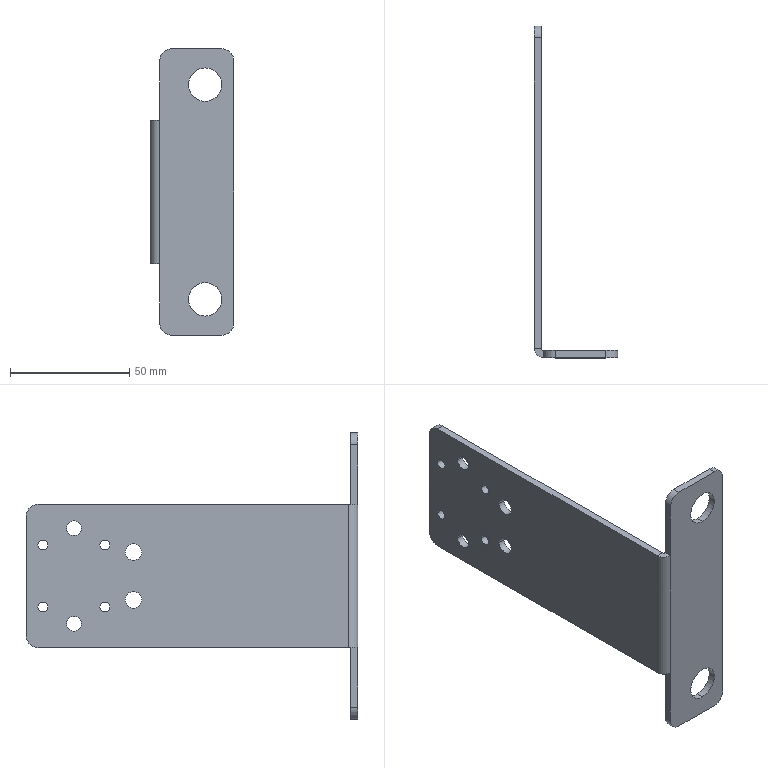Part | SolidWorks | features ICE 5, Fillet 2, ExtruThin 1, FlatPattern 1, FlattenBends 1, ProcessBends 1, SheetMetal 1 | 1 solid | 44 faces | box 35 x 139 x 120 mm | volume 34584 mm3 | cylinder 28 | plane 16 | commonest cylinder face diameters 4.2 x8 10 x6 6.2 x4 7 x4 14 x4 1.6 x1
STEP:
#1=CARTESIAN_POINT('',(0.,97.5,10.));
#2=VERTEX_POINT('',#1);
#3=CARTESIAN_POINT('',(0.,90.5,10.));
#4=VERTEX_POINT('',#3);
#5=CARTESIAN_POINT('',(0.,94.,10.));
#6=DIRECTION('',(-1.,0.,0.));
#7=DIRECTION('',(0.,-1.,0.));
#8=AXIS2_PLACEMENT_3D('',#5,#6,#7);
#9=CIRCLE('',#8,3.5);
#10=EDGE_CURVE('',#2,#4,#9,.T.);
#11=ORIENTED_EDGE('',*,*,#10,.T.);
#12=CARTESIAN_POINT('',(3.,90.5,10.));
#13=VERTEX_POINT('',#12);
#14=CARTESIAN_POINT('',(-7.,90.5,10.));
#15=DIRECTION('',(1.,0.,0.));
#16=VECTOR('',#15,1000.);
#17=LINE('',#14,#16);
#18=EDGE_CURVE('',#4,#13,#17,.T.);
#19=ORIENTED_EDGE('',*,*,#18,.T.);
#20=CARTESIAN_POINT('',(3.,97.5,10.));
#21=VERTEX_POINT('',#20);
#22=CARTESIAN_POINT('',(3.,94.,10.));
#23=DIRECTION('',(1.,0.,0.));
#24=DIRECTION('',(0.,1.,0.));
#25=AXIS2_PLACEMENT_3D('',#22,#23,#24);
#26=CIRCLE('',#25,3.5);
#27=EDGE_CURVE('',#13,#21,#26,.T.);
#28=ORIENTED_EDGE('',*,*,#27,.T.);
#29=CARTESIAN_POINT('',(-7.,97.5,10.));
#30=DIRECTION('',(1.,0.,0.));
#31=VECTOR('',#30,1000.);
#32=LINE('',#29,#31);
#33=EDGE_CURVE('',#2,#21,#32,.T.);
#34=ORIENTED_EDGE('',*,*,#33,.F.);
#35=EDGE_LOOP('',(#11,#19,#28,#34));
#36=FACE_OUTER_BOUND('',#35,.T.);
#37=CARTESIAN_POINT('',(-7.,94.,10.));
#38=DIRECTION('',(1.,0.,0.));
#39=DIRECTION('',(0.,1.,0.));
#40=AXIS2_PLACEMENT_3D('',#37,#38,#39);
#41=CYLINDRICAL_SURFACE('',#40,3.5);
#42=ADVANCED_FACE('',(#36),#41,.F.);
#43=CARTESIAN_POINT('',(0.,97.5,-10.));
#44=VERTEX_POINT('',#43);
#45=CARTESIAN_POINT('',(0.,90.5,-10.));
#46=VERTEX_POINT('',#45);
#47=CARTESIAN_POINT('',(0.,94.,-10.));
#48=DIRECTION('',(-1.,0.,0.));
#49=DIRECTION('',(0.,-1.,0.));
#50=AXIS2_PLACEMENT_3D('',#47,#48,#49);
#51=CIRCLE('',#50,3.5);
#52=EDGE_CURVE('',#44,#46,#51,.T.);
#53=ORIENTED_EDGE('',*,*,#52,.T.);
#54=CARTESIAN_POINT('',(3.,90.5,-10.));
#55=VERTEX_POINT('',#54);
#56=CARTESIAN_POINT('',(-7.,90.5,-10.));
#57=DIRECTION('',(1.,0.,0.));
#58=VECTOR('',#57,1000.);
#59=LINE('',#56,#58);
#60=EDGE_CURVE('',#46,#55,#59,.T.);
#61=ORIENTED_EDGE('',*,*,#60,.T.);
#62=CARTESIAN_POINT('',(3.,97.5,-10.));
#63=VERTEX_POINT('',#62);
#64=CARTESIAN_POINT('',(3.,94.,-10.));
#65=DIRECTION('',(1.,0.,0.));
#66=DIRECTION('',(0.,1.,0.));
#67=AXIS2_PLACEMENT_3D('',#64,#65,#66);
#68=CIRCLE('',#67,3.5);
#69=EDGE_CURVE('',#55,#63,#68,.T.);
#70=ORIENTED_EDGE('',*,*,#69,.T.);
#71=CARTESIAN_POINT('',(-7.,97.5,-10.));
#72=DIRECTION('',(1.,0.,0.));
#73=VECTOR('',#72,1000.);
#74=LINE('',#71,#73);
#75=EDGE_CURVE('',#44,#63,#74,.T.);
#76=ORIENTED_EDGE('',*,*,#75,.F.);
#77=EDGE_LOOP('',(#53,#61,#70,#76));
#78=FACE_OUTER_BOUND('',#77,.T.);
#79=CARTESIAN_POINT('',(-7.,94.,-10.));
#80=DIRECTION('',(1.,0.,0.));
#81=DIRECTION('',(0.,1.,0.));
#82=AXIS2_PLACEMENT_3D('',#79,#80,#81);
#83=CYLINDRICAL_SURFACE('',#82,3.5);
#84=ADVANCED_FACE('',(#78),#83,.F.);
#85=CARTESIAN_POINT('',(0.,122.1,-20.));
#86=VERTEX_POINT('',#85);
#87=CARTESIAN_POINT('',(0.,115.9,-20.));
#88=VERTEX_POINT('',#87);
#89=CARTESIAN_POINT('',(0.,119.,-20.));
#90=DIRECTION('',(-1.,0.,0.));
#91=DIRECTION('',(0.,-1.,0.));
#92=AXIS2_PLACEMENT_3D('',#89,#90,#91);
#93=CIRCLE('',#92,3.1);
#94=EDGE_CURVE('',#86,#88,#93,.T.);
#95=ORIENTED_EDGE('',*,*,#94,.T.);
#96=CARTESIAN_POINT('',(3.,115.9,-20.));
#97=VERTEX_POINT('',#96);
#98=CARTESIAN_POINT('',(-7.,115.9,-20.));
#99=DIRECTION('',(1.,0.,0.));
#100=VECTOR('',#99,1000.);
#101=LINE('',#98,#100);
#102=EDGE_CURVE('',#88,#97,#101,.T.);
#103=ORIENTED_EDGE('',*,*,#102,.T.);
#104=CARTESIAN_POINT('',(3.,122.1,-20.));
#105=VERTEX_POINT('',#104);
#106=CARTESIAN_POINT('',(3.,119.,-20.));
#107=DIRECTION('',(1.,0.,0.));
#108=DIRECTION('',(0.,1.,0.));
#109=AXIS2_PLACEMENT_3D('',#106,#107,#108);
#110=CIRCLE('',#109,3.1);
#111=EDGE_CURVE('',#97,#105,#110,.T.);
#112=ORIENTED_EDGE('',*,*,#111,.T.);
#113=CARTESIAN_POINT('',(-7.,122.1,-20.));
#114=DIRECTION('',(1.,0.,0.));
#115=VECTOR('',#114,1000.);
#116=LINE('',#113,#115);
#117=EDGE_CURVE('',#86,#105,#116,.T.);
#118=ORIENTED_EDGE('',*,*,#117,.F.);
#119=EDGE_LOOP('',(#95,#103,#112,#118));
#120=FACE_OUTER_BOUND('',#119,.T.);
#121=CARTESIAN_POINT('',(-7.,119.,-20.));
#122=DIRECTION('',(1.,0.,0.));
#123=DIRECTION('',(0.,1.,0.));
#124=AXIS2_PLACEMENT_3D('',#121,#122,#123);
#125=CYLINDRICAL_SURFACE('',#124,3.1);
#126=ADVANCED_FACE('',(#120),#125,.F.);
#127=CARTESIAN_POINT('',(0.,108.1,13.));
#128=VERTEX_POINT('',#127);
#129=CARTESIAN_POINT('',(0.,103.9,13.));
#130=VERTEX_POINT('',#129);
#131=CARTESIAN_POINT('',(0.,106.,13.));
#132=DIRECTION('',(-1.,0.,0.));
#133=DIRECTION('',(0.,-1.,0.));
#134=AXIS2_PLACEMENT_3D('',#131,#132,#133);
#135=CIRCLE('',#134,2.1);
#136=EDGE_CURVE('',#128,#130,#135,.T.);
#137=ORIENTED_EDGE('',*,*,#136,.T.);
#138=CARTESIAN_POINT('',(3.,103.9,13.));
#139=VERTEX_POINT('',#138);
#140=CARTESIAN_POINT('',(-7.,103.9,13.));
#141=DIRECTION('',(1.,0.,0.));
#142=VECTOR('',#141,1000.);
#143=LINE('',#140,#142);
#144=EDGE_CURVE('',#130,#139,#143,.T.);
#145=ORIENTED_EDGE('',*,*,#144,.T.);
#146=CARTESIAN_POINT('',(3.,108.1,13.));
#147=VERTEX_POINT('',#146);
#148=CARTESIAN_POINT('',(3.,106.,13.));
#149=DIRECTION('',(1.,0.,0.));
#150=DIRECTION('',(0.,1.,0.));
#151=AXIS2_PLACEMENT_3D('',#148,#149,#150);
#152=CIRCLE('',#151,2.1);
#153=EDGE_CURVE('',#139,#147,#152,.T.);
#154=ORIENTED_EDGE('',*,*,#153,.T.);
#155=CARTESIAN_POINT('',(-7.,108.1,13.));
#156=DIRECTION('',(1.,0.,0.));
#157=VECTOR('',#156,1000.);
#158=LINE('',#155,#157);
#159=EDGE_CURVE('',#128,#147,#158,.T.);
#160=ORIENTED_EDGE('',*,*,#159,.F.);
#161=EDGE_LOOP('',(#137,#145,#154,#160));
#162=FACE_OUTER_BOUND('',#161,.T.);
#163=CARTESIAN_POINT('',(-7.,106.,13.));
#164=DIRECTION('',(1.,0.,0.));
#165=DIRECTION('',(0.,1.,0.));
#166=AXIS2_PLACEMENT_3D('',#163,#164,#165);
#167=CYLINDRICAL_SURFACE('',#166,2.1);
#168=ADVANCED_FACE('',(#162),#167,.F.);
#169=CARTESIAN_POINT('',(0.,108.1,-13.));
#170=VERTEX_POINT('',#169);
#171=CARTESIAN_POINT('',(0.,103.9,-13.));
#172=VERTEX_POINT('',#171);
#173=CARTESIAN_POINT('',(0.,106.,-13.));
#174=DIRECTION('',(-1.,0.,0.));
#175=DIRECTION('',(0.,-1.,0.));
#176=AXIS2_PLACEMENT_3D('',#173,#174,#175);
#177=CIRCLE('',#176,2.1);
#178=EDGE_CURVE('',#170,#172,#177,.T.);
#179=ORIENTED_EDGE('',*,*,#178,.T.);
#180=CARTESIAN_POINT('',(3.,103.9,-13.));
#181=VERTEX_POINT('',#180);
#182=CARTESIAN_POINT('',(-7.,103.9,-13.));
#183=DIRECTION('',(1.,0.,0.));
#184=VECTOR('',#183,1000.);
#185=LINE('',#182,#184);
#186=EDGE_CURVE('',#172,#181,#185,.T.);
#187=ORIENTED_EDGE('',*,*,#186,.T.);
#188=CARTESIAN_POINT('',(3.,108.1,-13.));
#189=VERTEX_POINT('',#188);
#190=CARTESIAN_POINT('',(3.,106.,-13.));
#191=DIRECTION('',(1.,0.,0.));
#192=DIRECTION('',(0.,1.,0.));
#193=AXIS2_PLACEMENT_3D('',#190,#191,#192);
#194=CIRCLE('',#193,2.1);
#195=EDGE_CURVE('',#181,#189,#194,.T.);
#196=ORIENTED_EDGE('',*,*,#195,.T.);
#197=CARTESIAN_POINT('',(-7.,108.1,-13.));
#198=DIRECTION('',(1.,0.,0.));
#199=VECTOR('',#198,1000.);
#200=LINE('',#197,#199);
#201=EDGE_CURVE('',#170,#189,#200,.T.);
#202=ORIENTED_EDGE('',*,*,#201,.F.);
#203=EDGE_LOOP('',(#179,#187,#196,#202));
#204=FACE_OUTER_BOUND('',#203,.T.);
#205=CARTESIAN_POINT('',(-7.,106.,-13.));
#206=DIRECTION('',(1.,0.,0.));
#207=DIRECTION('',(0.,1.,0.));
#208=AXIS2_PLACEMENT_3D('',#205,#206,#207);
#209=CYLINDRICAL_SURFACE('',#208,2.1);
#210=ADVANCED_FACE('',(#204),#209,.F.);
#211=CARTESIAN_POINT('',(0.,134.1,-13.));
#212=VERTEX_POINT('',#211);
#213=CARTESIAN_POINT('',(0.,129.9,-13.));
#214=VERTEX_POINT('',#213);
#215=CARTESIAN_POINT('',(0.,132.,-13.));
#216=DIRECTION('',(-1.,0.,0.));
#217=DIRECTION('',(0.,-1.,0.));
#218=AXIS2_PLACEMENT_3D('',#215,#216,#217);
#219=CIRCLE('',#218,2.1);
#220=EDGE_CURVE('',#212,#214,#219,.T.);
#221=ORIENTED_EDGE('',*,*,#220,.T.);
#222=CARTESIAN_POINT('',(3.,129.9,-13.));
#223=VERTEX_POINT('',#222);
#224=CARTESIAN_POINT('',(-7.,129.9,-13.));
#225=DIRECTION('',(1.,0.,0.));
#226=VECTOR('',#225,1000.);
#227=LINE('',#224,#226);
#228=EDGE_CURVE('',#214,#223,#227,.T.);
#229=ORIENTED_EDGE('',*,*,#228,.T.);
#230=CARTESIAN_POINT('',(3.,134.1,-13.));
#231=VERTEX_POINT('',#230);
#232=CARTESIAN_POINT('',(3.,132.,-13.));
#233=DIRECTION('',(1.,0.,0.));
#234=DIRECTION('',(0.,1.,0.));
#235=AXIS2_PLACEMENT_3D('',#232,#233,#234);
#236=CIRCLE('',#235,2.1);
#237=EDGE_CURVE('',#223,#231,#236,.T.);
#238=ORIENTED_EDGE('',*,*,#237,.T.);
#239=CARTESIAN_POINT('',(-7.,134.1,-13.));
#240=DIRECTION('',(1.,0.,0.));
#241=VECTOR('',#240,1000.);
#242=LINE('',#239,#241);
#243=EDGE_CURVE('',#212,#231,#242,.T.);
#244=ORIENTED_EDGE('',*,*,#243,.F.);
#245=EDGE_LOOP('',(#221,#229,#238,#244));
#246=FACE_OUTER_BOUND('',#245,.T.);
#247=CARTESIAN_POINT('',(-7.,132.,-13.));
#248=DIRECTION('',(1.,0.,0.));
#249=DIRECTION('',(0.,1.,0.));
#250=AXIS2_PLACEMENT_3D('',#247,#248,#249);
#251=CYLINDRICAL_SURFACE('',#250,2.1);
#252=ADVANCED_FACE('',(#246),#251,.F.);
#253=CARTESIAN_POINT('',(0.,134.1,13.));
#254=VERTEX_POINT('',#253);
#255=CARTESIAN_POINT('',(0.,129.9,13.));
#256=VERTEX_POINT('',#255);
#257=CARTESIAN_POINT('',(0.,132.,13.));
#258=DIRECTION('',(-1.,0.,0.));
#259=DIRECTION('',(0.,-1.,0.));
#260=AXIS2_PLACEMENT_3D('',#257,#258,#259);
#261=CIRCLE('',#260,2.1);
#262=EDGE_CURVE('',#254,#256,#261,.T.);
#263=ORIENTED_EDGE('',*,*,#262,.T.);
#264=CARTESIAN_POINT('',(3.,129.9,13.));
#265=VERTEX_POINT('',#264);
#266=CARTESIAN_POINT('',(-7.,129.9,13.));
#267=DIRECTION('',(1.,0.,0.));
#268=VECTOR('',#267,1000.);
#269=LINE('',#266,#268);
#270=EDGE_CURVE('',#256,#265,#269,.T.);
#271=ORIENTED_EDGE('',*,*,#270,.T.);
#272=CARTESIAN_POINT('',(3.,134.1,13.));
#273=VERTEX_POINT('',#272);
#274=CARTESIAN_POINT('',(3.,132.,13.));
#275=DIRECTION('',(1.,0.,0.));
#276=DIRECTION('',(0.,1.,0.));
#277=AXIS2_PLACEMENT_3D('',#274,#275,#276);
#278=CIRCLE('',#277,2.1);
#279=EDGE_CURVE('',#265,#273,#278,.T.);
#280=ORIENTED_EDGE('',*,*,#279,.T.);
#281=CARTESIAN_POINT('',(-7.,134.1,13.));
#282=DIRECTION('',(1.,0.,0.));
#283=VECTOR('',#282,1000.);
#284=LINE('',#281,#283);
#285=EDGE_CURVE('',#254,#273,#284,.T.);
#286=ORIENTED_EDGE('',*,*,#285,.F.);
#287=EDGE_LOOP('',(#263,#271,#280,#286));
#288=FACE_OUTER_BOUND('',#287,.T.);
#289=CARTESIAN_POINT('',(-7.,132.,13.));
#290=DIRECTION('',(1.,0.,0.));
#291=DIRECTION('',(0.,1.,0.));
#292=AXIS2_PLACEMENT_3D('',#289,#290,#291);
#293=CYLINDRICAL_SURFACE('',#292,2.1);
#294=ADVANCED_FACE('',(#288),#293,.F.);
#295=CARTESIAN_POINT('',(0.,122.1,20.));
#296=VERTEX_POINT('',#295);
#297=CARTESIAN_POINT('',(0.,115.9,20.));
#298=VERTEX_POINT('',#297);
#299=CARTESIAN_POINT('',(0.,119.,20.));
#300=DIRECTION('',(-1.,0.,0.));
#301=DIRECTION('',(0.,-1.,0.));
#302=AXIS2_PLACEMENT_3D('',#299,#300,#301);
#303=CIRCLE('',#302,3.1);
#304=EDGE_CURVE('',#296,#298,#303,.T.);
#305=ORIENTED_EDGE('',*,*,#304,.T.);
#306=CARTESIAN_POINT('',(3.,115.9,20.));
#307=VERTEX_POINT('',#306);
#308=CARTESIAN_POINT('',(-7.,115.9,20.));
#309=DIRECTION('',(1.,0.,0.));
#310=VECTOR('',#309,1000.);
#311=LINE('',#308,#310);
#312=EDGE_CURVE('',#298,#307,#311,.T.);
#313=ORIENTED_EDGE('',*,*,#312,.T.);
#314=CARTESIAN_POINT('',(3.,122.1,20.));
#315=VERTEX_POINT('',#314);
#316=CARTESIAN_POINT('',(3.,119.,20.));
#317=DIRECTION('',(1.,0.,0.));
#318=DIRECTION('',(0.,1.,0.));
#319=AXIS2_PLACEMENT_3D('',#316,#317,#318);
#320=CIRCLE('',#319,3.1);
#321=EDGE_CURVE('',#307,#315,#320,.T.);
#322=ORIENTED_EDGE('',*,*,#321,.T.);
#323=CARTESIAN_POINT('',(-7.,122.1,20.));
#324=DIRECTION('',(1.,0.,0.));
#325=VECTOR('',#324,1000.);
#326=LINE('',#323,#325);
#327=EDGE_CURVE('',#296,#315,#326,.T.);
#328=ORIENTED_EDGE('',*,*,#327,.F.);
#329=EDGE_LOOP('',(#305,#313,#322,#328));
#330=FACE_OUTER_BOUND('',#329,.T.);
#331=CARTESIAN_POINT('',(-7.,119.,20.));
#332=DIRECTION('',(1.,0.,0.));
#333=DIRECTION('',(0.,1.,0.));
#334=AXIS2_PLACEMENT_3D('',#331,#332,#333);
#335=CYLINDRICAL_SURFACE('',#334,3.1);
#336=ADVANCED_FACE('',(#330),#335,.F.);
#337=CARTESIAN_POINT('',(23.,0.,-38.));
#338=VERTEX_POINT('',#337);
#339=CARTESIAN_POINT('',(23.,0.,-52.));
#340=VERTEX_POINT('',#339);
#341=CARTESIAN_POINT('',(23.,0.,-45.));
#342=DIRECTION('',(0.,-1.,0.));
#343=DIRECTION('',(0.,0.,-1.));
#344=AXIS2_PLACEMENT_3D('',#341,#342,#343);
#345=CIRCLE('',#344,7.);
#346=EDGE_CURVE('',#338,#340,#345,.T.);
#347=ORIENTED_EDGE('',*,*,#346,.T.);
#348=CARTESIAN_POINT('',(23.,3.,-52.));
#349=VERTEX_POINT('',#348);
#350=CARTESIAN_POINT('',(23.,-7.,-52.));
#351=DIRECTION('',(0.,1.,0.));
#352=VECTOR('',#351,1000.);
#353=LINE('',#350,#352);
#354=EDGE_CURVE('',#340,#349,#353,.T.);
#355=ORIENTED_EDGE('',*,*,#354,.T.);
#356=CARTESIAN_POINT('',(23.,3.,-38.));
#357=VERTEX_POINT('',#356);
#358=CARTESIAN_POINT('',(23.,3.,-45.));
#359=DIRECTION('',(0.,1.,0.));
#360=DIRECTION('',(0.,0.,1.));
#361=AXIS2_PLACEMENT_3D('',#358,#359,#360);
#362=CIRCLE('',#361,7.);
#363=EDGE_CURVE('',#349,#357,#362,.T.);
#364=ORIENTED_EDGE('',*,*,#363,.T.);
#365=CARTESIAN_POINT('',(23.,-7.,-38.));
#366=DIRECTION('',(0.,1.,0.));
#367=VECTOR('',#366,1000.);
#368=LINE('',#365,#367);
#369=EDGE_CURVE('',#338,#357,#368,.T.);
#370=ORIENTED_EDGE('',*,*,#369,.F.);
#371=EDGE_LOOP('',(#347,#355,#364,#370));
#372=FACE_OUTER_BOUND('',#371,.T.);
#373=CARTESIAN_POINT('',(23.,-7.,-45.));
#374=DIRECTION('',(0.,1.,0.));
#375=DIRECTION('',(0.,0.,1.));
#376=AXIS2_PLACEMENT_3D('',#373,#374,#375);
#377=CYLINDRICAL_SURFACE('',#376,7.);
#378=ADVANCED_FACE('',(#372),#377,.F.);
#379=CARTESIAN_POINT('',(23.,0.,52.));
#380=VERTEX_POINT('',#379);
#381=CARTESIAN_POINT('',(23.,0.,38.));
#382=VERTEX_POINT('',#381);
#383=CARTESIAN_POINT('',(23.,0.,45.));
#384=DIRECTION('',(0.,-1.,0.));
#385=DIRECTION('',(0.,0.,-1.));
#386=AXIS2_PLACEMENT_3D('',#383,#384,#385);
#387=CIRCLE('',#386,7.);
#388=EDGE_CURVE('',#380,#382,#387,.T.);
#389=ORIENTED_EDGE('',*,*,#388,.T.);
#390=CARTESIAN_POINT('',(23.,3.,38.));
#391=VERTEX_POINT('',#390);
#392=CARTESIAN_POINT('',(23.,-7.,38.));
#393=DIRECTION('',(0.,1.,0.));
#394=VECTOR('',#393,1000.);
#395=LINE('',#392,#394);
#396=EDGE_CURVE('',#382,#391,#395,.T.);
#397=ORIENTED_EDGE('',*,*,#396,.T.);
#398=CARTESIAN_POINT('',(23.,3.,52.));
#399=VERTEX_POINT('',#398);
#400=CARTESIAN_POINT('',(23.,3.,45.));
#401=DIRECTION('',(0.,1.,0.));
#402=DIRECTION('',(0.,0.,1.));
#403=AXIS2_PLACEMENT_3D('',#400,#401,#402);
#404=CIRCLE('',#403,7.);
#405=EDGE_CURVE('',#391,#399,#404,.T.);
#406=ORIENTED_EDGE('',*,*,#405,.T.);
#407=CARTESIAN_POINT('',(23.,-7.,52.));
#408=DIRECTION('',(0.,1.,0.));
#409=VECTOR('',#408,1000.);
#410=LINE('',#407,#409);
#411=EDGE_CURVE('',#380,#399,#410,.T.);
#412=ORIENTED_EDGE('',*,*,#411,.F.);
#413=EDGE_LOOP('',(#389,#397,#406,#412));
#414=FACE_OUTER_BOUND('',#413,.T.);
#415=CARTESIAN_POINT('',(23.,-7.,45.));
#416=DIRECTION('',(0.,1.,0.));
#417=DIRECTION('',(0.,0.,1.));
#418=AXIS2_PLACEMENT_3D('',#415,#416,#417);
#419=CYLINDRICAL_SURFACE('',#418,7.);
#420=ADVANCED_FACE('',(#414),#419,.F.);
#421=ORIENTED_EDGE('',*,*,#396,.F.);
#422=CARTESIAN_POINT('',(23.,0.,45.));
#423=DIRECTION('',(0.,-1.,0.));
#424=DIRECTION('',(0.,0.,-1.));
#425=AXIS2_PLACEMENT_3D('',#422,#423,#424);
#426=CIRCLE('',#425,7.);
#427=EDGE_CURVE('',#382,#380,#426,.T.);
#428=ORIENTED_EDGE('',*,*,#427,.T.);
#429=ORIENTED_EDGE('',*,*,#411,.T.);
#430=CARTESIAN_POINT('',(23.,3.,45.));
#431=DIRECTION('',(0.,1.,0.));
#432=DIRECTION('',(0.,0.,1.));
#433=AXIS2_PLACEMENT_3D('',#430,#431,#432);
#434=CIRCLE('',#433,7.);
#435=EDGE_CURVE('',#399,#391,#434,.T.);
#436=ORIENTED_EDGE('',*,*,#435,.T.);
#437=EDGE_LOOP('',(#421,#428,#429,#436));
#438=FACE_OUTER_BOUND('',#437,.T.);
#439=CARTESIAN_POINT('',(23.,-7.,45.));
#440=DIRECTION('',(0.,1.,0.));
#441=DIRECTION('',(0.,0.,1.));
#442=AXIS2_PLACEMENT_3D('',#439,#440,#441);
#443=CYLINDRICAL_SURFACE('',#442,7.);
#444=ADVANCED_FACE('',(#438),#443,.F.);
#445=ORIENTED_EDGE('',*,*,#354,.F.);
#446=CARTESIAN_POINT('',(23.,0.,-45.));
#447=DIRECTION('',(0.,-1.,0.));
#448=DIRECTION('',(0.,0.,-1.));
#449=AXIS2_PLACEMENT_3D('',#446,#447,#448);
#450=CIRCLE('',#449,7.);
#451=EDGE_CURVE('',#340,#338,#450,.T.);
#452=ORIENTED_EDGE('',*,*,#451,.T.);
#453=ORIENTED_EDGE('',*,*,#369,.T.);
#454=CARTESIAN_POINT('',(23.,3.,-45.));
#455=DIRECTION('',(0.,1.,0.));
#456=DIRECTION('',(0.,0.,1.));
#457=AXIS2_PLACEMENT_3D('',#454,#455,#456);
#458=CIRCLE('',#457,7.);
#459=EDGE_CURVE('',#357,#349,#458,.T.);
#460=ORIENTED_EDGE('',*,*,#459,.T.);
#461=EDGE_LOOP('',(#445,#452,#453,#460));
#462=FACE_OUTER_BOUND('',#461,.T.);
#463=CARTESIAN_POINT('',(23.,-7.,-45.));
#464=DIRECTION('',(0.,1.,0.));
#465=DIRECTION('',(0.,0.,1.));
#466=AXIS2_PLACEMENT_3D('',#463,#464,#465);
#467=CYLINDRICAL_SURFACE('',#466,7.);
#468=ADVANCED_FACE('',(#462),#467,.F.);
#469=CARTESIAN_POINT('',(9.,0.,60.));
#470=VERTEX_POINT('',#469);
#471=CARTESIAN_POINT('',(4.,0.,55.));
#472=VERTEX_POINT('',#471);
#473=CARTESIAN_POINT('',(9.,0.,55.));
#474=DIRECTION('',(0.,-1.,0.));
#475=DIRECTION('',(0.,0.,-1.));
#476=AXIS2_PLACEMENT_3D('',#473,#474,#475);
#477=CIRCLE('',#476,5.);
#478=EDGE_CURVE('',#470,#472,#477,.T.);
#479=ORIENTED_EDGE('',*,*,#478,.F.);
#480=CARTESIAN_POINT('',(9.,3.,60.));
#481=VERTEX_POINT('',#480);
#482=CARTESIAN_POINT('',(9.,247.979,60.));
#483=DIRECTION('',(0.,-1.,0.));
#484=VECTOR('',#483,1000.);
#485=LINE('',#482,#484);
#486=EDGE_CURVE('',#481,#470,#485,.T.);
#487=ORIENTED_EDGE('',*,*,#486,.F.);
#488=CARTESIAN_POINT('',(4.,3.,55.));
#489=VERTEX_POINT('',#488);
#490=CARTESIAN_POINT('',(9.,3.,55.));
#491=DIRECTION('',(0.,1.,0.));
#492=DIRECTION('',(0.,0.,-1.));
#493=AXIS2_PLACEMENT_3D('',#490,#491,#492);
#494=CIRCLE('',#493,5.);
#495=EDGE_CURVE('',#489,#481,#494,.T.);
#496=ORIENTED_EDGE('',*,*,#495,.F.);
#497=CARTESIAN_POINT('',(4.,247.979,55.));
#498=DIRECTION('',(0.,-1.,0.));
#499=VECTOR('',#498,1000.);
#500=LINE('',#497,#499);
#501=EDGE_CURVE('',#489,#472,#500,.T.);
#502=ORIENTED_EDGE('',*,*,#501,.T.);
#503=EDGE_LOOP('',(#479,#487,#496,#502));
#504=FACE_OUTER_BOUND('',#503,.T.);
#505=CARTESIAN_POINT('',(9.,247.979,55.));
#506=DIRECTION('',(0.,-1.,0.));
#507=DIRECTION('',(1.,0.,0.));
#508=AXIS2_PLACEMENT_3D('',#505,#506,#507);
#509=CYLINDRICAL_SURFACE('',#508,5.);
#510=ADVANCED_FACE('',(#504),#509,.T.);
#511=CARTESIAN_POINT('',(30.,0.,60.));
#512=VERTEX_POINT('',#511);
#513=CARTESIAN_POINT('',(0.,0.,60.));
#514=DIRECTION('',(1.,0.,0.));
#515=VECTOR('',#514,1000.);
#516=LINE('',#513,#515);
#517=EDGE_CURVE('',#470,#512,#516,.T.);
#518=ORIENTED_EDGE('',*,*,#517,.T.);
#519=CARTESIAN_POINT('',(30.,3.,60.));
#520=VERTEX_POINT('',#519);
#521=CARTESIAN_POINT('',(30.,247.979,60.));
#522=DIRECTION('',(0.,-1.,0.));
#523=VECTOR('',#522,1000.);
#524=LINE('',#521,#523);
#525=EDGE_CURVE('',#520,#512,#524,.T.);
#526=ORIENTED_EDGE('',*,*,#525,.F.);
#527=CARTESIAN_POINT('',(0.,3.,60.));
#528=DIRECTION('',(1.,0.,0.));
#529=VECTOR('',#528,1000.);
#530=LINE('',#527,#529);
#531=EDGE_CURVE('',#481,#520,#530,.T.);
#532=ORIENTED_EDGE('',*,*,#531,.F.);
#533=ORIENTED_EDGE('',*,*,#486,.T.);
#534=EDGE_LOOP('',(#518,#526,#532,#533));
#535=FACE_OUTER_BOUND('',#534,.T.);
#536=CARTESIAN_POINT('',(0.,247.979,60.));
#537=DIRECTION('',(0.,0.,-1.));
#538=DIRECTION('',(0.,-1.,0.));
#539=AXIS2_PLACEMENT_3D('',#536,#537,#538);
#540=PLANE('',#539);
#541=ADVANCED_FACE('',(#535),#540,.F.);
#542=CARTESIAN_POINT('',(35.,0.,55.));
#543=VERTEX_POINT('',#542);
#544=CARTESIAN_POINT('',(30.,0.,55.));
#545=DIRECTION('',(0.,-1.,0.));
#546=DIRECTION('',(0.,0.,-1.));
#547=AXIS2_PLACEMENT_3D('',#544,#545,#546);
#548=CIRCLE('',#547,5.);
#549=EDGE_CURVE('',#543,#512,#548,.T.);
#550=ORIENTED_EDGE('',*,*,#549,.F.);
#551=CARTESIAN_POINT('',(35.,3.,55.));
#552=VERTEX_POINT('',#551);
#553=CARTESIAN_POINT('',(35.,247.979,55.));
#554=DIRECTION('',(0.,-1.,0.));
#555=VECTOR('',#554,1000.);
#556=LINE('',#553,#555);
#557=EDGE_CURVE('',#552,#543,#556,.T.);
#558=ORIENTED_EDGE('',*,*,#557,.F.);
#559=CARTESIAN_POINT('',(30.,3.,55.));
#560=DIRECTION('',(0.,1.,0.));
#561=DIRECTION('',(0.,0.,-1.));
#562=AXIS2_PLACEMENT_3D('',#559,#560,#561);
#563=CIRCLE('',#562,5.);
#564=EDGE_CURVE('',#520,#552,#563,.T.);
#565=ORIENTED_EDGE('',*,*,#564,.F.);
#566=ORIENTED_EDGE('',*,*,#525,.T.);
#567=EDGE_LOOP('',(#550,#558,#565,#566));
#568=FACE_OUTER_BOUND('',#567,.T.);
#569=CARTESIAN_POINT('',(30.,247.979,55.));
#570=DIRECTION('',(0.,-1.,0.));
#571=DIRECTION('',(1.,0.,0.));
#572=AXIS2_PLACEMENT_3D('',#569,#570,#571);
#573=CYLINDRICAL_SURFACE('',#572,5.);
#574=ADVANCED_FACE('',(#568),#573,.T.);
#575=ORIENTED_EDGE('',*,*,#557,.T.);
#576=CARTESIAN_POINT('',(35.,0.,-55.));
#577=VERTEX_POINT('',#576);
#578=CARTESIAN_POINT('',(35.,0.,-60.));
#579=DIRECTION('',(0.,0.,1.));
#580=VECTOR('',#579,1000.);
#581=LINE('',#578,#580);
#582=EDGE_CURVE('',#577,#543,#581,.T.);
#583=ORIENTED_EDGE('',*,*,#582,.F.);
#584=CARTESIAN_POINT('',(35.,3.,-55.));
#585=VERTEX_POINT('',#584);
#586=CARTESIAN_POINT('',(35.,247.979,-55.));
#587=DIRECTION('',(0.,-1.,0.));
#588=VECTOR('',#587,1000.);
#589=LINE('',#586,#588);
#590=EDGE_CURVE('',#585,#577,#589,.T.);
#591=ORIENTED_EDGE('',*,*,#590,.F.);
#592=CARTESIAN_POINT('',(35.,3.,-60.));
#593=DIRECTION('',(0.,0.,1.));
#594=VECTOR('',#593,1000.);
#595=LINE('',#592,#594);
#596=EDGE_CURVE('',#585,#552,#595,.T.);
#597=ORIENTED_EDGE('',*,*,#596,.T.);
#598=EDGE_LOOP('',(#575,#583,#591,#597));
#599=FACE_OUTER_BOUND('',#598,.T.);
#600=CARTESIAN_POINT('',(35.,247.979,-60.));
#601=DIRECTION('',(1.,0.,0.));
#602=DIRECTION('',(0.,1.,0.));
#603=AXIS2_PLACEMENT_3D('',#600,#601,#602);
#604=PLANE('',#603);
#605=ADVANCED_FACE('',(#599),#604,.T.);
#606=CARTESIAN_POINT('',(30.,0.,-60.));
#607=VERTEX_POINT('',#606);
#608=CARTESIAN_POINT('',(30.,0.,-55.));
#609=DIRECTION('',(0.,-1.,0.));
#610=DIRECTION('',(0.,0.,-1.));
#611=AXIS2_PLACEMENT_3D('',#608,#609,#610);
#612=CIRCLE('',#611,5.);
#613=EDGE_CURVE('',#607,#577,#612,.T.);
#614=ORIENTED_EDGE('',*,*,#613,.F.);
#615=CARTESIAN_POINT('',(30.,3.,-60.));
#616=VERTEX_POINT('',#615);
#617=CARTESIAN_POINT('',(30.,247.979,-60.));
#618=DIRECTION('',(0.,-1.,0.));
#619=VECTOR('',#618,1000.);
#620=LINE('',#617,#619);
#621=EDGE_CURVE('',#616,#607,#620,.T.);
#622=ORIENTED_EDGE('',*,*,#621,.F.);
#623=CARTESIAN_POINT('',(30.,3.,-55.));
#624=DIRECTION('',(0.,1.,0.));
#625=DIRECTION('',(0.,0.,-1.));
#626=AXIS2_PLACEMENT_3D('',#623,#624,#625);
#627=CIRCLE('',#626,5.);
#628=EDGE_CURVE('',#585,#616,#627,.T.);
#629=ORIENTED_EDGE('',*,*,#628,.F.);
#630=ORIENTED_EDGE('',*,*,#590,.T.);
#631=EDGE_LOOP('',(#614,#622,#629,#630));
#632=FACE_OUTER_BOUND('',#631,.T.);
#633=CARTESIAN_POINT('',(30.,247.979,-55.));
#634=DIRECTION('',(0.,-1.,0.));
#635=DIRECTION('',(1.,0.,0.));
#636=AXIS2_PLACEMENT_3D('',#633,#634,#635);
#637=CYLINDRICAL_SURFACE('',#636,5.);
#638=ADVANCED_FACE('',(#632),#637,.T.);
#639=ORIENTED_EDGE('',*,*,#621,.T.);
#640=CARTESIAN_POINT('',(9.,0.,-60.));
#641=VERTEX_POINT('',#640);
#642=CARTESIAN_POINT('',(0.,0.,-60.));
#643=DIRECTION('',(1.,0.,0.));
#644=VECTOR('',#643,1000.);
#645=LINE('',#642,#644);
#646=EDGE_CURVE('',#641,#607,#645,.T.);
#647=ORIENTED_EDGE('',*,*,#646,.F.);
#648=CARTESIAN_POINT('',(9.,3.,-60.));
#649=VERTEX_POINT('',#648);
#650=CARTESIAN_POINT('',(9.,247.979,-60.));
#651=DIRECTION('',(0.,-1.,0.));
#652=VECTOR('',#651,1000.);
#653=LINE('',#650,#652);
#654=EDGE_CURVE('',#649,#641,#653,.T.);
#655=ORIENTED_EDGE('',*,*,#654,.F.);
#656=CARTESIAN_POINT('',(0.,3.,-60.));
#657=DIRECTION('',(1.,0.,0.));
#658=VECTOR('',#657,1000.);
#659=LINE('',#656,#658);
#660=EDGE_CURVE('',#649,#616,#659,.T.);
#661=ORIENTED_EDGE('',*,*,#660,.T.);
#662=EDGE_LOOP('',(#639,#647,#655,#661));
#663=FACE_OUTER_BOUND('',#662,.T.);
#664=CARTESIAN_POINT('',(0.,247.979,-60.));
#665=DIRECTION('',(0.,0.,-1.));
#666=DIRECTION('',(0.,-1.,0.));
#667=AXIS2_PLACEMENT_3D('',#664,#665,#666);
#668=PLANE('',#667);
#669=ADVANCED_FACE('',(#663),#668,.T.);
#670=CARTESIAN_POINT('',(4.,0.,-55.));
#671=VERTEX_POINT('',#670);
#672=CARTESIAN_POINT('',(9.,0.,-55.));
#673=DIRECTION('',(0.,-1.,0.));
#674=DIRECTION('',(0.,0.,-1.));
#675=AXIS2_PLACEMENT_3D('',#672,#673,#674);
#676=CIRCLE('',#675,5.);
#677=EDGE_CURVE('',#671,#641,#676,.T.);
#678=ORIENTED_EDGE('',*,*,#677,.F.);
#679=CARTESIAN_POINT('',(4.,3.,-55.));
#680=VERTEX_POINT('',#679);
#681=CARTESIAN_POINT('',(4.,247.979,-55.));
#682=DIRECTION('',(0.,-1.,0.));
#683=VECTOR('',#682,1000.);
#684=LINE('',#681,#683);
#685=EDGE_CURVE('',#680,#671,#684,.T.);
#686=ORIENTED_EDGE('',*,*,#685,.F.);
#687=CARTESIAN_POINT('',(9.,3.,-55.));
#688=DIRECTION('',(0.,1.,0.));
#689=DIRECTION('',(0.,0.,-1.));
#690=AXIS2_PLACEMENT_3D('',#687,#688,#689);
#691=CIRCLE('',#690,5.);
#692=EDGE_CURVE('',#649,#680,#691,.T.);
#693=ORIENTED_EDGE('',*,*,#692,.F.);
#694=ORIENTED_EDGE('',*,*,#654,.T.);
#695=EDGE_LOOP('',(#678,#686,#693,#694));
#696=FACE_OUTER_BOUND('',#695,.T.);
#697=CARTESIAN_POINT('',(9.,247.979,-55.));
#698=DIRECTION('',(0.,-1.,0.));
#699=DIRECTION('',(1.,0.,0.));
#700=AXIS2_PLACEMENT_3D('',#697,#698,#699);
#701=CYLINDRICAL_SURFACE('',#700,5.);
#702=ADVANCED_FACE('',(#696),#701,.T.);
#703=ORIENTED_EDGE('',*,*,#685,.T.);
#704=CARTESIAN_POINT('',(4.,0.,-30.));
#705=VERTEX_POINT('',#704);
#706=CARTESIAN_POINT('',(4.,0.,-60.));
#707=DIRECTION('',(0.,0.,1.));
#708=VECTOR('',#707,1000.);
#709=LINE('',#706,#708);
#710=EDGE_CURVE('',#671,#705,#709,.T.);
#711=ORIENTED_EDGE('',*,*,#710,.T.);
#712=CARTESIAN_POINT('',(4.,3.,-30.));
#713=VERTEX_POINT('',#712);
#714=CARTESIAN_POINT('',(4.,247.979,-30.));
#715=DIRECTION('',(0.,-1.,0.));
#716=VECTOR('',#715,1000.);
#717=LINE('',#714,#716);
#718=EDGE_CURVE('',#713,#705,#717,.T.);
#719=ORIENTED_EDGE('',*,*,#718,.F.);
#720=CARTESIAN_POINT('',(4.,3.,-30.));
#721=DIRECTION('',(0.,0.,-1.));
#722=VECTOR('',#721,1000.);
#723=LINE('',#720,#722);
#724=EDGE_CURVE('',#713,#680,#723,.T.);
#725=ORIENTED_EDGE('',*,*,#724,.T.);
#726=EDGE_LOOP('',(#703,#711,#719,#725));
#727=FACE_OUTER_BOUND('',#726,.T.);
#728=CARTESIAN_POINT('',(4.,247.979,-30.));
#729=DIRECTION('',(-1.,0.,0.));
#730=DIRECTION('',(0.,-1.,0.));
#731=AXIS2_PLACEMENT_3D('',#728,#729,#730);
#732=PLANE('',#731);
#733=ADVANCED_FACE('',(#727),#732,.T.);
#734=CARTESIAN_POINT('',(4.,3.,30.));
#735=VERTEX_POINT('',#734);
#736=CARTESIAN_POINT('',(4.,0.,30.));
#737=VERTEX_POINT('',#736);
#738=CARTESIAN_POINT('',(4.,247.979,30.));
#739=DIRECTION('',(0.,-1.,0.));
#740=VECTOR('',#739,1000.);
#741=LINE('',#738,#740);
#742=EDGE_CURVE('',#735,#737,#741,.T.);
#743=ORIENTED_EDGE('',*,*,#742,.T.);
#744=CARTESIAN_POINT('',(4.,0.,-60.));
#745=DIRECTION('',(0.,0.,1.));
#746=VECTOR('',#745,1000.);
#747=LINE('',#744,#746);
#748=EDGE_CURVE('',#737,#472,#747,.T.);
#749=ORIENTED_EDGE('',*,*,#748,.T.);
#750=ORIENTED_EDGE('',*,*,#501,.F.);
#751=CARTESIAN_POINT('',(4.,3.,30.));
#752=DIRECTION('',(0.,0.,-1.));
#753=VECTOR('',#752,1000.);
#754=LINE('',#751,#753);
#755=EDGE_CURVE('',#489,#735,#754,.T.);
#756=ORIENTED_EDGE('',*,*,#755,.T.);
#757=EDGE_LOOP('',(#743,#749,#750,#756));
#758=FACE_OUTER_BOUND('',#757,.T.);
#759=CARTESIAN_POINT('',(4.,247.979,30.));
#760=DIRECTION('',(-1.,0.,0.));
#761=DIRECTION('',(0.,0.,1.));
#762=AXIS2_PLACEMENT_3D('',#759,#760,#761);
#763=PLANE('',#762);
#764=ADVANCED_FACE('',(#758),#763,.T.);
#765=CARTESIAN_POINT('',(3.8,3.,30.));
#766=VERTEX_POINT('',#765);
#767=CARTESIAN_POINT('',(3.8,0.,30.));
#768=VERTEX_POINT('',#767);
#769=CARTESIAN_POINT('',(3.8,247.979,30.));
#770=DIRECTION('',(0.,-1.,0.));
#771=VECTOR('',#770,1000.);
#772=LINE('',#769,#771);
#773=EDGE_CURVE('',#766,#768,#772,.T.);
#774=ORIENTED_EDGE('',*,*,#773,.T.);
#775=CARTESIAN_POINT('',(0.,0.,30.));
#776=DIRECTION('',(1.,0.,0.));
#777=VECTOR('',#776,1000.);
#778=LINE('',#775,#777);
#779=EDGE_CURVE('',#768,#737,#778,.T.);
#780=ORIENTED_EDGE('',*,*,#779,.T.);
#781=ORIENTED_EDGE('',*,*,#742,.F.);
#782=CARTESIAN_POINT('',(4.,3.,30.));
#783=DIRECTION('',(-1.,0.,0.));
#784=VECTOR('',#783,1000.);
#785=LINE('',#782,#784);
#786=EDGE_CURVE('',#735,#766,#785,.T.);
#787=ORIENTED_EDGE('',*,*,#786,.T.);
#788=EDGE_LOOP('',(#774,#780,#781,#787));
#789=FACE_OUTER_BOUND('',#788,.T.);
#790=CARTESIAN_POINT('',(4.,247.979,30.));
#791=DIRECTION('',(0.,0.,1.));
#792=DIRECTION('',(0.,1.,0.));
#793=AXIS2_PLACEMENT_3D('',#790,#791,#792);
#794=PLANE('',#793);
#795=ADVANCED_FACE('',(#789),#794,.T.);
#796=CARTESIAN_POINT('',(3.8,0.,-30.));
#797=VERTEX_POINT('',#796);
#798=CARTESIAN_POINT('',(3.8,0.,30.));
#799=DIRECTION('',(0.,0.,1.));
#800=VECTOR('',#799,1000.);
#801=LINE('',#798,#800);
#802=EDGE_CURVE('',#797,#768,#801,.T.);
#803=ORIENTED_EDGE('',*,*,#802,.F.);
#804=CARTESIAN_POINT('',(0.,0.,-30.));
#805=DIRECTION('',(-1.,0.,0.));
#806=VECTOR('',#805,1000.);
#807=LINE('',#804,#806);
#808=EDGE_CURVE('',#705,#797,#807,.T.);
#809=ORIENTED_EDGE('',*,*,#808,.F.);
#810=ORIENTED_EDGE('',*,*,#710,.F.);
#811=ORIENTED_EDGE('',*,*,#677,.T.);
#812=ORIENTED_EDGE('',*,*,#646,.T.);
#813=ORIENTED_EDGE('',*,*,#613,.T.);
#814=ORIENTED_EDGE('',*,*,#582,.T.);
#815=ORIENTED_EDGE('',*,*,#549,.T.);
#816=ORIENTED_EDGE('',*,*,#517,.F.);
#817=ORIENTED_EDGE('',*,*,#478,.T.);
#818=ORIENTED_EDGE('',*,*,#748,.F.);
#819=ORIENTED_EDGE('',*,*,#779,.F.);
#820=EDGE_LOOP('',(#803,#809,#810,#811,#812,#813,#814,#815,#816,#817,#818,#819));
#821=FACE_OUTER_BOUND('',#820,.T.);
#822=ORIENTED_EDGE('',*,*,#346,.F.);
#823=ORIENTED_EDGE('',*,*,#451,.F.);
#824=EDGE_LOOP('',(#822,#823));
#825=FACE_BOUND('',#824,.T.);
#826=ORIENTED_EDGE('',*,*,#388,.F.);
#827=ORIENTED_EDGE('',*,*,#427,.F.);
#828=EDGE_LOOP('',(#826,#827));
#829=FACE_BOUND('',#828,.T.);
#830=CARTESIAN_POINT('',(0.,0.,-60.));
#831=DIRECTION('',(0.,-1.,0.));
#832=DIRECTION('',(0.,0.,-1.));
#833=AXIS2_PLACEMENT_3D('',#830,#831,#832);
#834=PLANE('',#833);
#835=ADVANCED_FACE('',(#821,#825,#829),#834,.T.);
#836=ORIENTED_EDGE('',*,*,#718,.T.);
#837=ORIENTED_EDGE('',*,*,#808,.T.);
#838=CARTESIAN_POINT('',(3.8,3.,-30.));
#839=VERTEX_POINT('',#838);
#840=CARTESIAN_POINT('',(3.8,247.979,-30.));
#841=DIRECTION('',(0.,-1.,0.));
#842=VECTOR('',#841,1000.);
#843=LINE('',#840,#842);
#844=EDGE_CURVE('',#839,#797,#843,.T.);
#845=ORIENTED_EDGE('',*,*,#844,.F.);
#846=CARTESIAN_POINT('',(4.,3.,-30.));
#847=DIRECTION('',(-1.,0.,0.));
#848=VECTOR('',#847,1000.);
#849=LINE('',#846,#848);
#850=EDGE_CURVE('',#713,#839,#849,.T.);
#851=ORIENTED_EDGE('',*,*,#850,.F.);
#852=EDGE_LOOP('',(#836,#837,#845,#851));
#853=FACE_OUTER_BOUND('',#852,.T.);
#854=CARTESIAN_POINT('',(4.,247.979,-30.));
#855=DIRECTION('',(0.,0.,-1.));
#856=DIRECTION('',(0.,-1.,0.));
#857=AXIS2_PLACEMENT_3D('',#854,#855,#856);
#858=PLANE('',#857);
#859=ADVANCED_FACE('',(#853),#858,.T.);
#860=ORIENTED_EDGE('',*,*,#459,.F.);
#861=ORIENTED_EDGE('',*,*,#363,.F.);
#862=EDGE_LOOP('',(#860,#861));
#863=FACE_BOUND('',#862,.T.);
#864=ORIENTED_EDGE('',*,*,#435,.F.);
#865=ORIENTED_EDGE('',*,*,#405,.F.);
#866=EDGE_LOOP('',(#864,#865));
#867=FACE_BOUND('',#866,.T.);
#868=ORIENTED_EDGE('',*,*,#850,.T.);
#869=CARTESIAN_POINT('',(3.8,3.,30.));
#870=DIRECTION('',(0.,0.,1.));
#871=VECTOR('',#870,1000.);
#872=LINE('',#869,#871);
#873=EDGE_CURVE('',#839,#766,#872,.T.);
#874=ORIENTED_EDGE('',*,*,#873,.T.);
#875=ORIENTED_EDGE('',*,*,#786,.F.);
#876=ORIENTED_EDGE('',*,*,#755,.F.);
#877=ORIENTED_EDGE('',*,*,#495,.T.);
#878=ORIENTED_EDGE('',*,*,#531,.T.);
#879=ORIENTED_EDGE('',*,*,#564,.T.);
#880=ORIENTED_EDGE('',*,*,#596,.F.);
#881=ORIENTED_EDGE('',*,*,#628,.T.);
#882=ORIENTED_EDGE('',*,*,#660,.F.);
#883=ORIENTED_EDGE('',*,*,#692,.T.);
#884=ORIENTED_EDGE('',*,*,#724,.F.);
#885=EDGE_LOOP('',(#868,#874,#875,#876,#877,#878,#879,#880,#881,#882,#883,#884));
#886=FACE_OUTER_BOUND('',#885,.T.);
#887=CARTESIAN_POINT('',(0.,3.,-60.));
#888=DIRECTION('',(0.,-1.,0.));
#889=DIRECTION('',(0.,0.,-1.));
#890=AXIS2_PLACEMENT_3D('',#887,#888,#889);
#891=PLANE('',#890);
#892=ADVANCED_FACE('',(#863,#867,#886),#891,.F.);
#893=ORIENTED_EDGE('',*,*,#10,.F.);
#894=CARTESIAN_POINT('',(0.,94.,10.));
#895=DIRECTION('',(-1.,0.,0.));
#896=DIRECTION('',(0.,-1.,0.));
#897=AXIS2_PLACEMENT_3D('',#894,#895,#896);
#898=CIRCLE('',#897,3.5);
#899=EDGE_CURVE('',#4,#2,#898,.T.);
#900=ORIENTED_EDGE('',*,*,#899,.F.);
#901=EDGE_LOOP('',(#893,#900));
#902=FACE_BOUND('',#901,.T.);
#903=ORIENTED_EDGE('',*,*,#52,.F.);
#904=CARTESIAN_POINT('',(0.,94.,-10.));
#905=DIRECTION('',(-1.,0.,0.));
#906=DIRECTION('',(0.,-1.,0.));
#907=AXIS2_PLACEMENT_3D('',#904,#905,#906);
#908=CIRCLE('',#907,3.5);
#909=EDGE_CURVE('',#46,#44,#908,.T.);
#910=ORIENTED_EDGE('',*,*,#909,.F.);
#911=EDGE_LOOP('',(#903,#910));
#912=FACE_BOUND('',#911,.T.);
#913=ORIENTED_EDGE('',*,*,#94,.F.);
#914=CARTESIAN_POINT('',(0.,119.,-20.));
#915=DIRECTION('',(-1.,0.,0.));
#916=DIRECTION('',(0.,-1.,0.));
#917=AXIS2_PLACEMENT_3D('',#914,#915,#916);
#918=CIRCLE('',#917,3.1);
#919=EDGE_CURVE('',#88,#86,#918,.T.);
#920=ORIENTED_EDGE('',*,*,#919,.F.);
#921=EDGE_LOOP('',(#913,#920));
#922=FACE_BOUND('',#921,.T.);
#923=ORIENTED_EDGE('',*,*,#136,.F.);
#924=CARTESIAN_POINT('',(0.,106.,13.));
#925=DIRECTION('',(-1.,0.,0.));
#926=DIRECTION('',(0.,-1.,0.));
#927=AXIS2_PLACEMENT_3D('',#924,#925,#926);
#928=CIRCLE('',#927,2.1);
#929=EDGE_CURVE('',#130,#128,#928,.T.);
#930=ORIENTED_EDGE('',*,*,#929,.F.);
#931=EDGE_LOOP('',(#923,#930));
#932=FACE_BOUND('',#931,.T.);
#933=ORIENTED_EDGE('',*,*,#178,.F.);
#934=CARTESIAN_POINT('',(0.,106.,-13.));
#935=DIRECTION('',(-1.,0.,0.));
#936=DIRECTION('',(0.,-1.,0.));
#937=AXIS2_PLACEMENT_3D('',#934,#935,#936);
#938=CIRCLE('',#937,2.1);
#939=EDGE_CURVE('',#172,#170,#938,.T.);
#940=ORIENTED_EDGE('',*,*,#939,.F.);
#941=EDGE_LOOP('',(#933,#940));
#942=FACE_BOUND('',#941,.T.);
#943=ORIENTED_EDGE('',*,*,#220,.F.);
#944=CARTESIAN_POINT('',(0.,132.,-13.));
#945=DIRECTION('',(-1.,0.,0.));
#946=DIRECTION('',(0.,-1.,0.));
#947=AXIS2_PLACEMENT_3D('',#944,#945,#946);
#948=CIRCLE('',#947,2.1);
#949=EDGE_CURVE('',#214,#212,#948,.T.);
#950=ORIENTED_EDGE('',*,*,#949,.F.);
#951=EDGE_LOOP('',(#943,#950));
#952=FACE_BOUND('',#951,.T.);
#953=ORIENTED_EDGE('',*,*,#262,.F.);
#954=CARTESIAN_POINT('',(0.,132.,13.));
#955=DIRECTION('',(-1.,0.,0.));
#956=DIRECTION('',(0.,-1.,0.));
#957=AXIS2_PLACEMENT_3D('',#954,#955,#956);
#958=CIRCLE('',#957,2.1);
#959=EDGE_CURVE('',#256,#254,#958,.T.);
#960=ORIENTED_EDGE('',*,*,#959,.F.);
#961=EDGE_LOOP('',(#953,#960));
#962=FACE_BOUND('',#961,.T.);
#963=ORIENTED_EDGE('',*,*,#304,.F.);
#964=CARTESIAN_POINT('',(0.,119.,20.));
#965=DIRECTION('',(-1.,0.,0.));
#966=DIRECTION('',(0.,-1.,0.));
#967=AXIS2_PLACEMENT_3D('',#964,#965,#966);
#968=CIRCLE('',#967,3.1);
#969=EDGE_CURVE('',#298,#296,#968,.T.);
#970=ORIENTED_EDGE('',*,*,#969,.F.);
#971=EDGE_LOOP('',(#963,#970));
#972=FACE_BOUND('',#971,.T.);
#973=CARTESIAN_POINT('',(0.,3.8,-30.));
#974=VERTEX_POINT('',#973);
#975=CARTESIAN_POINT('',(0.,134.,-30.));
#976=VERTEX_POINT('',#975);
#977=CARTESIAN_POINT('',(0.,139.,-30.));
#978=DIRECTION('',(0.,1.,0.));
#979=VECTOR('',#978,1000.);
#980=LINE('',#977,#979);
#981=EDGE_CURVE('',#974,#976,#980,.T.);
#982=ORIENTED_EDGE('',*,*,#981,.F.);
#983=CARTESIAN_POINT('',(0.,3.8,30.));
#984=VERTEX_POINT('',#983);
#985=CARTESIAN_POINT('',(0.,3.8,30.));
#986=DIRECTION('',(0.,0.,1.));
#987=VECTOR('',#986,1000.);
#988=LINE('',#985,#987);
#989=EDGE_CURVE('',#974,#984,#988,.T.);
#990=ORIENTED_EDGE('',*,*,#989,.T.);
#991=CARTESIAN_POINT('',(0.,134.,30.));
#992=VERTEX_POINT('',#991);
#993=CARTESIAN_POINT('',(0.,139.,30.));
#994=DIRECTION('',(0.,-1.,0.));
#995=VECTOR('',#994,1000.);
#996=LINE('',#993,#995);
#997=EDGE_CURVE('',#992,#984,#996,.T.);
#998=ORIENTED_EDGE('',*,*,#997,.F.);
#999=CARTESIAN_POINT('',(0.,139.,25.));
#1000=VERTEX_POINT('',#999);
#1001=CARTESIAN_POINT('',(0.,134.,25.));
#1002=DIRECTION('',(-1.,0.,0.));
#1003=DIRECTION('',(0.,-1.,0.));
#1004=AXIS2_PLACEMENT_3D('',#1001,#1002,#1003);
#1005=CIRCLE('',#1004,5.);
#1006=EDGE_CURVE('',#992,#1000,#1005,.T.);
#1007=ORIENTED_EDGE('',*,*,#1006,.T.);
#1008=CARTESIAN_POINT('',(0.,139.,-25.));
#1009=VERTEX_POINT('',#1008);
#1010=CARTESIAN_POINT('',(0.,139.,-60.));
#1011=DIRECTION('',(0.,0.,1.));
#1012=VECTOR('',#1011,1000.);
#1013=LINE('',#1010,#1012);
#1014=EDGE_CURVE('',#1009,#1000,#1013,.T.);
#1015=ORIENTED_EDGE('',*,*,#1014,.F.);
#1016=CARTESIAN_POINT('',(0.,134.,-25.));
#1017=DIRECTION('',(-1.,0.,0.));
#1018=DIRECTION('',(0.,-1.,0.));
#1019=AXIS2_PLACEMENT_3D('',#1016,#1017,#1018);
#1020=CIRCLE('',#1019,5.);
#1021=EDGE_CURVE('',#1009,#976,#1020,.T.);
#1022=ORIENTED_EDGE('',*,*,#1021,.T.);
#1023=EDGE_LOOP('',(#982,#990,#998,#1007,#1015,#1022));
#1024=FACE_OUTER_BOUND('',#1023,.T.);
#1025=CARTESIAN_POINT('',(0.,139.,-60.));
#1026=DIRECTION('',(-1.,0.,0.));
#1027=DIRECTION('',(0.,-1.,0.));
#1028=AXIS2_PLACEMENT_3D('',#1025,#1026,#1027);
#1029=PLANE('',#1028);
#1030=ADVANCED_FACE('',(#902,#912,#922,#932,#942,#952,#962,#972,#1024),#1029,.T.);
#1031=CARTESIAN_POINT('',(3.,94.,10.));
#1032=DIRECTION('',(1.,0.,0.));
#1033=DIRECTION('',(0.,1.,0.));
#1034=AXIS2_PLACEMENT_3D('',#1031,#1032,#1033);
#1035=CIRCLE('',#1034,3.5);
#1036=EDGE_CURVE('',#21,#13,#1035,.T.);
#1037=ORIENTED_EDGE('',*,*,#1036,.F.);
#1038=ORIENTED_EDGE('',*,*,#27,.F.);
#1039=EDGE_LOOP('',(#1037,#1038));
#1040=FACE_BOUND('',#1039,.T.);
#1041=CARTESIAN_POINT('',(3.,94.,-10.));
#1042=DIRECTION('',(1.,0.,0.));
#1043=DIRECTION('',(0.,1.,0.));
#1044=AXIS2_PLACEMENT_3D('',#1041,#1042,#1043);
#1045=CIRCLE('',#1044,3.5);
#1046=EDGE_CURVE('',#63,#55,#1045,.T.);
#1047=ORIENTED_EDGE('',*,*,#1046,.F.);
#1048=ORIENTED_EDGE('',*,*,#69,.F.);
#1049=EDGE_LOOP('',(#1047,#1048));
#1050=FACE_BOUND('',#1049,.T.);
#1051=CARTESIAN_POINT('',(3.,119.,20.));
#1052=DIRECTION('',(1.,0.,0.));
#1053=DIRECTION('',(0.,1.,0.));
#1054=AXIS2_PLACEMENT_3D('',#1051,#1052,#1053);
#1055=CIRCLE('',#1054,3.1);
#1056=EDGE_CURVE('',#315,#307,#1055,.T.);
#1057=ORIENTED_EDGE('',*,*,#1056,.F.);
#1058=ORIENTED_EDGE('',*,*,#321,.F.);
#1059=EDGE_LOOP('',(#1057,#1058));
#1060=FACE_BOUND('',#1059,.T.);
#1061=CARTESIAN_POINT('',(3.,132.,13.));
#1062=DIRECTION('',(1.,0.,0.));
#1063=DIRECTION('',(0.,1.,0.));
#1064=AXIS2_PLACEMENT_3D('',#1061,#1062,#1063);
#1065=CIRCLE('',#1064,2.1);
#1066=EDGE_CURVE('',#273,#265,#1065,.T.);
#1067=ORIENTED_EDGE('',*,*,#1066,.F.);
#1068=ORIENTED_EDGE('',*,*,#279,.F.);
#1069=EDGE_LOOP('',(#1067,#1068));
#1070=FACE_BOUND('',#1069,.T.);
#1071=CARTESIAN_POINT('',(3.,132.,-13.));
#1072=DIRECTION('',(1.,0.,0.));
#1073=DIRECTION('',(0.,1.,0.));
#1074=AXIS2_PLACEMENT_3D('',#1071,#1072,#1073);
#1075=CIRCLE('',#1074,2.1);
#1076=EDGE_CURVE('',#231,#223,#1075,.T.);
#1077=ORIENTED_EDGE('',*,*,#1076,.F.);
#1078=ORIENTED_EDGE('',*,*,#237,.F.);
#1079=EDGE_LOOP('',(#1077,#1078));
#1080=FACE_BOUND('',#1079,.T.);
#1081=CARTESIAN_POINT('',(3.,106.,-13.));
#1082=DIRECTION('',(1.,0.,0.));
#1083=DIRECTION('',(0.,1.,0.));
#1084=AXIS2_PLACEMENT_3D('',#1081,#1082,#1083);
#1085=CIRCLE('',#1084,2.1);
#1086=EDGE_CURVE('',#189,#181,#1085,.T.);
#1087=ORIENTED_EDGE('',*,*,#1086,.F.);
#1088=ORIENTED_EDGE('',*,*,#195,.F.);
#1089=EDGE_LOOP('',(#1087,#1088));
#1090=FACE_BOUND('',#1089,.T.);
#1091=CARTESIAN_POINT('',(3.,106.,13.));
#1092=DIRECTION('',(1.,0.,0.));
#1093=DIRECTION('',(0.,1.,0.));
#1094=AXIS2_PLACEMENT_3D('',#1091,#1092,#1093);
#1095=CIRCLE('',#1094,2.1);
#1096=EDGE_CURVE('',#147,#139,#1095,.T.);
#1097=ORIENTED_EDGE('',*,*,#1096,.F.);
#1098=ORIENTED_EDGE('',*,*,#153,.F.);
#1099=EDGE_LOOP('',(#1097,#1098));
#1100=FACE_BOUND('',#1099,.T.);
#1101=CARTESIAN_POINT('',(3.,119.,-20.));
#1102=DIRECTION('',(1.,0.,0.));
#1103=DIRECTION('',(0.,1.,0.));
#1104=AXIS2_PLACEMENT_3D('',#1101,#1102,#1103);
#1105=CIRCLE('',#1104,3.1);
#1106=EDGE_CURVE('',#105,#97,#1105,.T.);
#1107=ORIENTED_EDGE('',*,*,#1106,.F.);
#1108=ORIENTED_EDGE('',*,*,#111,.F.);
#1109=EDGE_LOOP('',(#1107,#1108));
#1110=FACE_BOUND('',#1109,.T.);
#1111=CARTESIAN_POINT('',(3.,3.8,-30.));
#1112=VERTEX_POINT('',#1111);
#1113=CARTESIAN_POINT('',(3.,3.8,30.));
#1114=VERTEX_POINT('',#1113);
#1115=CARTESIAN_POINT('',(3.,3.8,30.));
#1116=DIRECTION('',(0.,0.,1.));
#1117=VECTOR('',#1116,1000.);
#1118=LINE('',#1115,#1117);
#1119=EDGE_CURVE('',#1112,#1114,#1118,.T.);
#1120=ORIENTED_EDGE('',*,*,#1119,.F.);
#1121=CARTESIAN_POINT('',(3.,134.,-30.));
#1122=VERTEX_POINT('',#1121);
#1123=CARTESIAN_POINT('',(3.,139.,-30.));
#1124=DIRECTION('',(0.,-1.,0.));
#1125=VECTOR('',#1124,1000.);
#1126=LINE('',#1123,#1125);
#1127=EDGE_CURVE('',#1122,#1112,#1126,.T.);
#1128=ORIENTED_EDGE('',*,*,#1127,.F.);
#1129=CARTESIAN_POINT('',(3.,139.,-25.));
#1130=VERTEX_POINT('',#1129);
#1131=CARTESIAN_POINT('',(3.,134.,-25.));
#1132=DIRECTION('',(1.,0.,0.));
#1133=DIRECTION('',(0.,-1.,0.));
#1134=AXIS2_PLACEMENT_3D('',#1131,#1132,#1133);
#1135=CIRCLE('',#1134,5.);
#1136=EDGE_CURVE('',#1122,#1130,#1135,.T.);
#1137=ORIENTED_EDGE('',*,*,#1136,.T.);
#1138=CARTESIAN_POINT('',(3.,139.,25.));
#1139=VERTEX_POINT('',#1138);
#1140=CARTESIAN_POINT('',(3.,139.,-60.));
#1141=DIRECTION('',(0.,0.,1.));
#1142=VECTOR('',#1141,1000.);
#1143=LINE('',#1140,#1142);
#1144=EDGE_CURVE('',#1130,#1139,#1143,.T.);
#1145=ORIENTED_EDGE('',*,*,#1144,.T.);
#1146=CARTESIAN_POINT('',(3.,134.,30.));
#1147=VERTEX_POINT('',#1146);
#1148=CARTESIAN_POINT('',(3.,134.,25.));
#1149=DIRECTION('',(1.,0.,0.));
#1150=DIRECTION('',(0.,-1.,0.));
#1151=AXIS2_PLACEMENT_3D('',#1148,#1149,#1150);
#1152=CIRCLE('',#1151,5.);
#1153=EDGE_CURVE('',#1139,#1147,#1152,.T.);
#1154=ORIENTED_EDGE('',*,*,#1153,.T.);
#1155=CARTESIAN_POINT('',(3.,139.,30.));
#1156=DIRECTION('',(0.,1.,0.));
#1157=VECTOR('',#1156,1000.);
#1158=LINE('',#1155,#1157);
#1159=EDGE_CURVE('',#1114,#1147,#1158,.T.);
#1160=ORIENTED_EDGE('',*,*,#1159,.F.);
#1161=EDGE_LOOP('',(#1120,#1128,#1137,#1145,#1154,#1160));
#1162=FACE_OUTER_BOUND('',#1161,.T.);
#1163=CARTESIAN_POINT('',(3.,139.,-60.));
#1164=DIRECTION('',(-1.,0.,0.));
#1165=DIRECTION('',(0.,-1.,0.));
#1166=AXIS2_PLACEMENT_3D('',#1163,#1164,#1165);
#1167=PLANE('',#1166);
#1168=ADVANCED_FACE('',(#1040,#1050,#1060,#1070,#1080,#1090,#1100,#1110,#1162),#1167,.F.);
#1169=ORIENTED_EDGE('',*,*,#312,.F.);
#1170=ORIENTED_EDGE('',*,*,#969,.T.);
#1171=ORIENTED_EDGE('',*,*,#327,.T.);
#1172=ORIENTED_EDGE('',*,*,#1056,.T.);
#1173=EDGE_LOOP('',(#1169,#1170,#1171,#1172));
#1174=FACE_OUTER_BOUND('',#1173,.T.);
#1175=CARTESIAN_POINT('',(-7.,119.,20.));
#1176=DIRECTION('',(1.,0.,0.));
#1177=DIRECTION('',(0.,1.,0.));
#1178=AXIS2_PLACEMENT_3D('',#1175,#1176,#1177);
#1179=CYLINDRICAL_SURFACE('',#1178,3.1);
#1180=ADVANCED_FACE('',(#1174),#1179,.F.);
#1181=ORIENTED_EDGE('',*,*,#270,.F.);
#1182=ORIENTED_EDGE('',*,*,#959,.T.);
#1183=ORIENTED_EDGE('',*,*,#285,.T.);
#1184=ORIENTED_EDGE('',*,*,#1066,.T.);
#1185=EDGE_LOOP('',(#1181,#1182,#1183,#1184));
#1186=FACE_OUTER_BOUND('',#1185,.T.);
#1187=CARTESIAN_POINT('',(-7.,132.,13.));
#1188=DIRECTION('',(1.,0.,0.));
#1189=DIRECTION('',(0.,1.,0.));
#1190=AXIS2_PLACEMENT_3D('',#1187,#1188,#1189);
#1191=CYLINDRICAL_SURFACE('',#1190,2.1);
#1192=ADVANCED_FACE('',(#1186),#1191,.F.);
#1193=ORIENTED_EDGE('',*,*,#228,.F.);
#1194=ORIENTED_EDGE('',*,*,#949,.T.);
#1195=ORIENTED_EDGE('',*,*,#243,.T.);
#1196=ORIENTED_EDGE('',*,*,#1076,.T.);
#1197=EDGE_LOOP('',(#1193,#1194,#1195,#1196));
#1198=FACE_OUTER_BOUND('',#1197,.T.);
#1199=CARTESIAN_POINT('',(-7.,132.,-13.));
#1200=DIRECTION('',(1.,0.,0.));
#1201=DIRECTION('',(0.,1.,0.));
#1202=AXIS2_PLACEMENT_3D('',#1199,#1200,#1201);
#1203=CYLINDRICAL_SURFACE('',#1202,2.1);
#1204=ADVANCED_FACE('',(#1198),#1203,.F.);
#1205=ORIENTED_EDGE('',*,*,#186,.F.);
#1206=ORIENTED_EDGE('',*,*,#939,.T.);
#1207=ORIENTED_EDGE('',*,*,#201,.T.);
#1208=ORIENTED_EDGE('',*,*,#1086,.T.);
#1209=EDGE_LOOP('',(#1205,#1206,#1207,#1208));
#1210=FACE_OUTER_BOUND('',#1209,.T.);
#1211=CARTESIAN_POINT('',(-7.,106.,-13.));
#1212=DIRECTION('',(1.,0.,0.));
#1213=DIRECTION('',(0.,1.,0.));
#1214=AXIS2_PLACEMENT_3D('',#1211,#1212,#1213);
#1215=CYLINDRICAL_SURFACE('',#1214,2.1);
#1216=ADVANCED_FACE('',(#1210),#1215,.F.);
#1217=ORIENTED_EDGE('',*,*,#144,.F.);
#1218=ORIENTED_EDGE('',*,*,#929,.T.);
#1219=ORIENTED_EDGE('',*,*,#159,.T.);
#1220=ORIENTED_EDGE('',*,*,#1096,.T.);
#1221=EDGE_LOOP('',(#1217,#1218,#1219,#1220));
#1222=FACE_OUTER_BOUND('',#1221,.T.);
#1223=CARTESIAN_POINT('',(-7.,106.,13.));
#1224=DIRECTION('',(1.,0.,0.));
#1225=DIRECTION('',(0.,1.,0.));
#1226=AXIS2_PLACEMENT_3D('',#1223,#1224,#1225);
#1227=CYLINDRICAL_SURFACE('',#1226,2.1);
#1228=ADVANCED_FACE('',(#1222),#1227,.F.);
#1229=ORIENTED_EDGE('',*,*,#102,.F.);
#1230=ORIENTED_EDGE('',*,*,#919,.T.);
#1231=ORIENTED_EDGE('',*,*,#117,.T.);
#1232=ORIENTED_EDGE('',*,*,#1106,.T.);
#1233=EDGE_LOOP('',(#1229,#1230,#1231,#1232));
#1234=FACE_OUTER_BOUND('',#1233,.T.);
#1235=CARTESIAN_POINT('',(-7.,119.,-20.));
#1236=DIRECTION('',(1.,0.,0.));
#1237=DIRECTION('',(0.,1.,0.));
#1238=AXIS2_PLACEMENT_3D('',#1235,#1236,#1237);
#1239=CYLINDRICAL_SURFACE('',#1238,3.1);
#1240=ADVANCED_FACE('',(#1234),#1239,.F.);
#1241=CARTESIAN_POINT('',(295.831,134.,30.));
#1242=DIRECTION('',(-1.,0.,0.));
#1243=VECTOR('',#1242,1000.);
#1244=LINE('',#1241,#1243);
#1245=EDGE_CURVE('',#1147,#992,#1244,.T.);
#1246=ORIENTED_EDGE('',*,*,#1245,.T.);
#1247=ORIENTED_EDGE('',*,*,#997,.T.);
#1248=CARTESIAN_POINT('',(295.831,3.8,30.));
#1249=DIRECTION('',(-1.,0.,0.));
#1250=VECTOR('',#1249,1000.);
#1251=LINE('',#1248,#1250);
#1252=EDGE_CURVE('',#1114,#984,#1251,.T.);
#1253=ORIENTED_EDGE('',*,*,#1252,.F.);
#1254=ORIENTED_EDGE('',*,*,#1159,.T.);
#1255=EDGE_LOOP('',(#1246,#1247,#1253,#1254));
#1256=FACE_OUTER_BOUND('',#1255,.T.);
#1257=CARTESIAN_POINT('',(295.831,139.,30.));
#1258=DIRECTION('',(0.,0.,1.));
#1259=DIRECTION('',(0.,-1.,0.));
#1260=AXIS2_PLACEMENT_3D('',#1257,#1258,#1259);
#1261=PLANE('',#1260);
#1262=ADVANCED_FACE('',(#1256),#1261,.T.);
#1263=CARTESIAN_POINT('',(295.831,3.8,-30.));
#1264=DIRECTION('',(-1.,0.,0.));
#1265=VECTOR('',#1264,1000.);
#1266=LINE('',#1263,#1265);
#1267=EDGE_CURVE('',#1112,#974,#1266,.T.);
#1268=ORIENTED_EDGE('',*,*,#1267,.T.);
#1269=ORIENTED_EDGE('',*,*,#981,.T.);
#1270=CARTESIAN_POINT('',(295.831,134.,-30.));
#1271=DIRECTION('',(-1.,0.,0.));
#1272=VECTOR('',#1271,1000.);
#1273=LINE('',#1270,#1272);
#1274=EDGE_CURVE('',#1122,#976,#1273,.T.);
#1275=ORIENTED_EDGE('',*,*,#1274,.F.);
#1276=ORIENTED_EDGE('',*,*,#1127,.T.);
#1277=EDGE_LOOP('',(#1268,#1269,#1275,#1276));
#1278=FACE_OUTER_BOUND('',#1277,.T.);
#1279=CARTESIAN_POINT('',(295.831,139.,-30.));
#1280=DIRECTION('',(0.,0.,-1.));
#1281=DIRECTION('',(0.,1.,0.));
#1282=AXIS2_PLACEMENT_3D('',#1279,#1280,#1281);
#1283=PLANE('',#1282);
#1284=ADVANCED_FACE('',(#1278),#1283,.T.);
#1285=ORIENTED_EDGE('',*,*,#1021,.F.);
#1286=CARTESIAN_POINT('',(295.831,139.,-25.));
#1287=DIRECTION('',(-1.,0.,0.));
#1288=VECTOR('',#1287,1000.);
#1289=LINE('',#1286,#1288);
#1290=EDGE_CURVE('',#1130,#1009,#1289,.T.);
#1291=ORIENTED_EDGE('',*,*,#1290,.F.);
#1292=ORIENTED_EDGE('',*,*,#1136,.F.);
#1293=ORIENTED_EDGE('',*,*,#1274,.T.);
#1294=EDGE_LOOP('',(#1285,#1291,#1292,#1293));
#1295=FACE_OUTER_BOUND('',#1294,.T.);
#1296=CARTESIAN_POINT('',(295.831,134.,-25.));
#1297=DIRECTION('',(-1.,0.,0.));
#1298=DIRECTION('',(0.,-1.,0.));
#1299=AXIS2_PLACEMENT_3D('',#1296,#1297,#1298);
#1300=CYLINDRICAL_SURFACE('',#1299,5.);
#1301=ADVANCED_FACE('',(#1295),#1300,.T.);
#1302=ORIENTED_EDGE('',*,*,#1014,.T.);
#1303=CARTESIAN_POINT('',(295.831,139.,25.));
#1304=DIRECTION('',(-1.,0.,0.));
#1305=VECTOR('',#1304,1000.);
#1306=LINE('',#1303,#1305);
#1307=EDGE_CURVE('',#1139,#1000,#1306,.T.);
#1308=ORIENTED_EDGE('',*,*,#1307,.F.);
#1309=ORIENTED_EDGE('',*,*,#1144,.F.);
#1310=ORIENTED_EDGE('',*,*,#1290,.T.);
#1311=EDGE_LOOP('',(#1302,#1308,#1309,#1310));
#1312=FACE_OUTER_BOUND('',#1311,.T.);
#1313=CARTESIAN_POINT('',(295.831,139.,-60.));
#1314=DIRECTION('',(0.,-1.,0.));
#1315=DIRECTION('',(1.,0.,0.));
#1316=AXIS2_PLACEMENT_3D('',#1313,#1314,#1315);
#1317=PLANE('',#1316);
#1318=ADVANCED_FACE('',(#1312),#1317,.F.);
#1319=ORIENTED_EDGE('',*,*,#1006,.F.);
#1320=ORIENTED_EDGE('',*,*,#1245,.F.);
#1321=ORIENTED_EDGE('',*,*,#1153,.F.);
#1322=ORIENTED_EDGE('',*,*,#1307,.T.);
#1323=EDGE_LOOP('',(#1319,#1320,#1321,#1322));
#1324=FACE_OUTER_BOUND('',#1323,.T.);
#1325=CARTESIAN_POINT('',(295.831,134.,25.));
#1326=DIRECTION('',(-1.,0.,0.));
#1327=DIRECTION('',(0.,-1.,0.));
#1328=AXIS2_PLACEMENT_3D('',#1325,#1326,#1327);
#1329=CYLINDRICAL_SURFACE('',#1328,5.);
#1330=ADVANCED_FACE('',(#1324),#1329,.T.);
#1331=ORIENTED_EDGE('',*,*,#773,.F.);
#1332=CARTESIAN_POINT('',(3.8,3.8,30.));
#1333=DIRECTION('',(0.,0.,-1.));
#1334=DIRECTION('',(0.,1.,0.));
#1335=AXIS2_PLACEMENT_3D('',#1332,#1333,#1334);
#1336=CIRCLE('',#1335,0.8);
#1337=EDGE_CURVE('',#766,#1114,#1336,.T.);
#1338=ORIENTED_EDGE('',*,*,#1337,.T.);
#1339=ORIENTED_EDGE('',*,*,#1252,.T.);
#1340=CARTESIAN_POINT('',(3.8,3.8,30.));
#1341=DIRECTION('',(0.,0.,-1.));
#1342=DIRECTION('',(0.,1.,0.));
#1343=AXIS2_PLACEMENT_3D('',#1340,#1341,#1342);
#1344=CIRCLE('',#1343,3.8);
#1345=EDGE_CURVE('',#768,#984,#1344,.T.);
#1346=ORIENTED_EDGE('',*,*,#1345,.F.);
#1347=EDGE_LOOP('',(#1331,#1338,#1339,#1346));
#1348=FACE_OUTER_BOUND('',#1347,.T.);
#1349=CARTESIAN_POINT('',(3.8,3.8,30.));
#1350=DIRECTION('',(0.,0.,1.));
#1351=DIRECTION('',(1.,0.,0.));
#1352=AXIS2_PLACEMENT_3D('',#1349,#1350,#1351);
#1353=PLANE('',#1352);
#1354=ADVANCED_FACE('',(#1348),#1353,.T.);
#1355=CARTESIAN_POINT('',(3.8,3.8,-30.));
#1356=DIRECTION('',(0.,0.,1.));
#1357=DIRECTION('',(0.,1.,0.));
#1358=AXIS2_PLACEMENT_3D('',#1355,#1356,#1357);
#1359=CIRCLE('',#1358,0.8);
#1360=EDGE_CURVE('',#1112,#839,#1359,.T.);
#1361=ORIENTED_EDGE('',*,*,#1360,.T.);
#1362=ORIENTED_EDGE('',*,*,#844,.T.);
#1363=CARTESIAN_POINT('',(3.8,3.8,-30.));
#1364=DIRECTION('',(0.,0.,1.));
#1365=DIRECTION('',(0.,1.,0.));
#1366=AXIS2_PLACEMENT_3D('',#1363,#1364,#1365);
#1367=CIRCLE('',#1366,3.8);
#1368=EDGE_CURVE('',#974,#797,#1367,.T.);
#1369=ORIENTED_EDGE('',*,*,#1368,.F.);
#1370=ORIENTED_EDGE('',*,*,#1267,.F.);
#1371=EDGE_LOOP('',(#1361,#1362,#1369,#1370));
#1372=FACE_OUTER_BOUND('',#1371,.T.);
#1373=CARTESIAN_POINT('',(3.8,3.8,-30.));
#1374=DIRECTION('',(0.,0.,-1.));
#1375=DIRECTION('',(-1.,0.,0.));
#1376=AXIS2_PLACEMENT_3D('',#1373,#1374,#1375);
#1377=PLANE('',#1376);
#1378=ADVANCED_FACE('',(#1372),#1377,.T.);
#1379=ORIENTED_EDGE('',*,*,#989,.F.);
#1380=ORIENTED_EDGE('',*,*,#1368,.T.);
#1381=ORIENTED_EDGE('',*,*,#802,.T.);
#1382=ORIENTED_EDGE('',*,*,#1345,.T.);
#1383=EDGE_LOOP('',(#1379,#1380,#1381,#1382));
#1384=FACE_OUTER_BOUND('',#1383,.T.);
#1385=CARTESIAN_POINT('',(3.8,3.8,237.157));
#1386=DIRECTION('',(0.,0.,-1.));
#1387=DIRECTION('',(0.,1.,0.));
#1388=AXIS2_PLACEMENT_3D('',#1385,#1386,#1387);
#1389=CYLINDRICAL_SURFACE('',#1388,3.8);
#1390=ADVANCED_FACE('',(#1384),#1389,.T.);
#1391=ORIENTED_EDGE('',*,*,#1119,.T.);
#1392=ORIENTED_EDGE('',*,*,#1337,.F.);
#1393=ORIENTED_EDGE('',*,*,#873,.F.);
#1394=ORIENTED_EDGE('',*,*,#1360,.F.);
#1395=EDGE_LOOP('',(#1391,#1392,#1393,#1394));
#1396=FACE_OUTER_BOUND('',#1395,.T.);
#1397=CARTESIAN_POINT('',(3.8,3.8,237.157));
#1398=DIRECTION('',(0.,0.,-1.));
#1399=DIRECTION('',(0.,1.,0.));
#1400=AXIS2_PLACEMENT_3D('',#1397,#1398,#1399);
#1401=CYLINDRICAL_SURFACE('',#1400,0.8);
#1402=ADVANCED_FACE('',(#1396),#1401,.F.);
#1403=ORIENTED_EDGE('',*,*,#60,.F.);
#1404=ORIENTED_EDGE('',*,*,#909,.T.);
#1405=ORIENTED_EDGE('',*,*,#75,.T.);
#1406=ORIENTED_EDGE('',*,*,#1046,.T.);
#1407=EDGE_LOOP('',(#1403,#1404,#1405,#1406));
#1408=FACE_OUTER_BOUND('',#1407,.T.);
#1409=CARTESIAN_POINT('',(-7.,94.,-10.));
#1410=DIRECTION('',(1.,0.,0.));
#1411=DIRECTION('',(0.,1.,0.));
#1412=AXIS2_PLACEMENT_3D('',#1409,#1410,#1411);
#1413=CYLINDRICAL_SURFACE('',#1412,3.5);
#1414=ADVANCED_FACE('',(#1408),#1413,.F.);
#1415=ORIENTED_EDGE('',*,*,#18,.F.);
#1416=ORIENTED_EDGE('',*,*,#899,.T.);
#1417=ORIENTED_EDGE('',*,*,#33,.T.);
#1418=ORIENTED_EDGE('',*,*,#1036,.T.);
#1419=EDGE_LOOP('',(#1415,#1416,#1417,#1418));
#1420=FACE_OUTER_BOUND('',#1419,.T.);
#1421=CARTESIAN_POINT('',(-7.,94.,10.));
#1422=DIRECTION('',(1.,0.,0.));
#1423=DIRECTION('',(0.,1.,0.));
#1424=AXIS2_PLACEMENT_3D('',#1421,#1422,#1423);
#1425=CYLINDRICAL_SURFACE('',#1424,3.5);
#1426=ADVANCED_FACE('',(#1420),#1425,.F.);
#1427=CLOSED_SHELL('',(#42,#84,#126,#168,#210,#252,#294,#336,#378,#420,#444,#468,#510,#541,#574,#605,#638,#669,#702,#733,#764,#795,#835,#859,#892,#1030,#1168,#1180,#1192,#1204,#1216,#1228,#1240,#1262,#1284,#1301,#1318,#1330,#1354,#1378,#1390,#1402,#1414,#1426));
#1428=MANIFOLD_SOLID_BREP('',#1427);
#1429=CARTESIAN_POINT('',(0.,0.,0.));
#1430=DIRECTION('',(0.,0.,1.));
#1431=DIRECTION('',(1.,0.,0.));
#1432=AXIS2_PLACEMENT_3D('',#1429,#1430,#1431);
#1433=(LENGTH_UNIT()NAMED_UNIT(*)SI_UNIT(.MILLI.,.METRE.));
#1434=UNCERTAINTY_MEASURE_WITH_UNIT(LENGTH_MEASURE(0.00001),#1433,'','');
#1435=(NAMED_UNIT(*)PLANE_ANGLE_UNIT()SI_UNIT($,.RADIAN.));
#1436=(NAMED_UNIT(*)SI_UNIT($,.STERADIAN.)SOLID_ANGLE_UNIT());
#1437=(GEOMETRIC_REPRESENTATION_CONTEXT(3)GLOBAL_UNCERTAINTY_ASSIGNED_CONTEXT((#1434))GLOBAL_UNIT_ASSIGNED_CONTEXT((#1433,#1435,#1436))REPRESENTATION_CONTEXT('',''));
#1438=ADVANCED_BREP_SHAPE_REPRESENTATION('',(#1428,#1432),#1437);